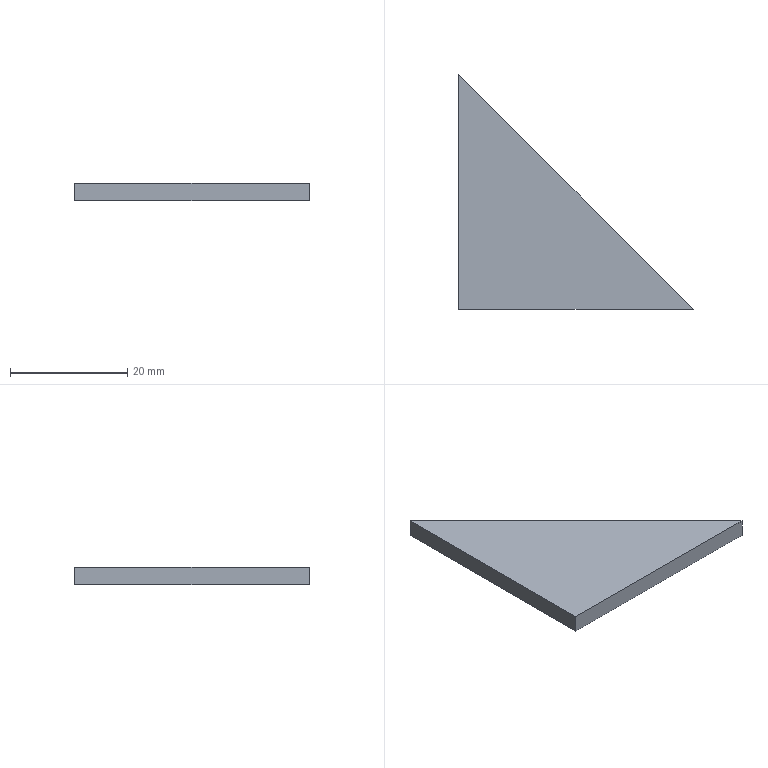Part | STEP file | 7100107 | 1 solid | 5 faces | box 40 x 40 x 3 mm | volume 2400 mm3 | plane 5
STEP:
#1=CARTESIAN_POINT('',(0.,0.,0.));
#2=DIRECTION('',(0.,0.,1.));
#3=DIRECTION('',(1.,0.,0.));
#4=AXIS2_PLACEMENT_3D('',#1,#2,#3);
#5=CARTESIAN_POINT('',(40.,-40.,0.));
#6=VERTEX_POINT('',#5);
#7=CARTESIAN_POINT('',(0.,0.,0.));
#8=VERTEX_POINT('',#7);
#9=CARTESIAN_POINT('',(40.,-40.,0.));
#10=DIRECTION('',(-0.7071,0.7071,0.));
#11=VECTOR('',#10,1.);
#12=LINE('',#9,#11);
#13=CARTESIAN_POINT('',(40.,-40.,3.));
#14=DIRECTION('',(-0.7071,-0.7071,0.));
#15=DIRECTION('',(0.7071,-0.7071,0.));
#16=AXIS2_PLACEMENT_3D('',#13,#14,#15);
#17=PLANE('',#16);
#18=CARTESIAN_POINT('',(0.,-3.));
#19=DIRECTION('',(-1.,0.));
#20=VECTOR('',#19,1.);
#21=LINE('',#18,#20);
#22=(GEOMETRIC_REPRESENTATION_CONTEXT(2)PARAMETRIC_REPRESENTATION_CONTEXT()REPRESENTATION_CONTEXT('',''));
#23=DEFINITIONAL_REPRESENTATION('',(#21),#22);
#24=PCURVE('',#17,#23);
#25=CARTESIAN_POINT('',(0.,0.,0.));
#26=DIRECTION('',(0.,0.,1.));
#27=DIRECTION('',(1.,0.,0.));
#28=AXIS2_PLACEMENT_3D('',#25,#26,#27);
#29=PLANE('',#28);
#30=CARTESIAN_POINT('',(40.,-40.));
#31=DIRECTION('',(-0.7071,0.7071));
#32=VECTOR('',#31,1.);
#33=LINE('',#30,#32);
#34=(GEOMETRIC_REPRESENTATION_CONTEXT(2)PARAMETRIC_REPRESENTATION_CONTEXT()REPRESENTATION_CONTEXT('',''));
#35=DEFINITIONAL_REPRESENTATION('',(#33),#34);
#36=PCURVE('',#29,#35);
#37=SURFACE_CURVE('',#12,(#24,#36),.PCURVE_S1.);
#38=EDGE_CURVE('',#6,#8,#37,.T.);
#39=ORIENTED_EDGE('',*,*,#38,.T.);
#40=CARTESIAN_POINT('',(0.,0.,3.));
#41=VERTEX_POINT('',#40);
#42=CARTESIAN_POINT('',(0.,0.,3.));
#43=DIRECTION('',(0.,0.,-1.));
#44=VECTOR('',#43,1.);
#45=LINE('',#42,#44);
#46=CARTESIAN_POINT('',(-56.569,0.));
#47=DIRECTION('',(0.,-1.));
#48=VECTOR('',#47,1.);
#49=LINE('',#46,#48);
#50=(GEOMETRIC_REPRESENTATION_CONTEXT(2)PARAMETRIC_REPRESENTATION_CONTEXT()REPRESENTATION_CONTEXT('',''));
#51=DEFINITIONAL_REPRESENTATION('',(#49),#50);
#52=PCURVE('',#17,#51);
#53=CARTESIAN_POINT('',(0.,0.,3.));
#54=DIRECTION('',(1.,0.,0.));
#55=DIRECTION('',(0.,1.,0.));
#56=AXIS2_PLACEMENT_3D('',#53,#54,#55);
#57=PLANE('',#56);
#58=CARTESIAN_POINT('',(0.,0.));
#59=DIRECTION('',(0.,-1.));
#60=VECTOR('',#59,1.);
#61=LINE('',#58,#60);
#62=(GEOMETRIC_REPRESENTATION_CONTEXT(2)PARAMETRIC_REPRESENTATION_CONTEXT()REPRESENTATION_CONTEXT('',''));
#63=DEFINITIONAL_REPRESENTATION('',(#61),#62);
#64=PCURVE('',#57,#63);
#65=SURFACE_CURVE('',#45,(#52,#64),.PCURVE_S1.);
#66=EDGE_CURVE('',#41,#8,#65,.T.);
#67=ORIENTED_EDGE('',*,*,#66,.F.);
#68=CARTESIAN_POINT('',(40.,-40.,3.));
#69=VERTEX_POINT('',#68);
#70=CARTESIAN_POINT('',(40.,-40.,3.));
#71=DIRECTION('',(-0.7071,0.7071,0.));
#72=VECTOR('',#71,1.);
#73=LINE('',#70,#72);
#74=CARTESIAN_POINT('',(0.,0.));
#75=DIRECTION('',(-1.,0.));
#76=VECTOR('',#75,1.);
#77=LINE('',#74,#76);
#78=(GEOMETRIC_REPRESENTATION_CONTEXT(2)PARAMETRIC_REPRESENTATION_CONTEXT()REPRESENTATION_CONTEXT('',''));
#79=DEFINITIONAL_REPRESENTATION('',(#77),#78);
#80=PCURVE('',#17,#79);
#81=CARTESIAN_POINT('',(0.,0.,3.));
#82=DIRECTION('',(0.,0.,1.));
#83=DIRECTION('',(1.,0.,0.));
#84=AXIS2_PLACEMENT_3D('',#81,#82,#83);
#85=PLANE('',#84);
#86=CARTESIAN_POINT('',(40.,-40.));
#87=DIRECTION('',(-0.7071,0.7071));
#88=VECTOR('',#87,1.);
#89=LINE('',#86,#88);
#90=(GEOMETRIC_REPRESENTATION_CONTEXT(2)PARAMETRIC_REPRESENTATION_CONTEXT()REPRESENTATION_CONTEXT('',''));
#91=DEFINITIONAL_REPRESENTATION('',(#89),#90);
#92=PCURVE('',#85,#91);
#93=SURFACE_CURVE('',#73,(#80,#92),.PCURVE_S1.);
#94=EDGE_CURVE('',#69,#41,#93,.T.);
#95=ORIENTED_EDGE('',*,*,#94,.F.);
#96=CARTESIAN_POINT('',(40.,-40.,3.));
#97=DIRECTION('',(0.,0.,-1.));
#98=VECTOR('',#97,1.);
#99=LINE('',#96,#98);
#100=CARTESIAN_POINT('',(0.,0.));
#101=DIRECTION('',(0.,-1.));
#102=VECTOR('',#101,1.);
#103=LINE('',#100,#102);
#104=(GEOMETRIC_REPRESENTATION_CONTEXT(2)PARAMETRIC_REPRESENTATION_CONTEXT()REPRESENTATION_CONTEXT('',''));
#105=DEFINITIONAL_REPRESENTATION('',(#103),#104);
#106=PCURVE('',#17,#105);
#107=CARTESIAN_POINT('',(0.,-40.,3.));
#108=DIRECTION('',(0.,1.,0.));
#109=DIRECTION('',(0.,0.,1.));
#110=AXIS2_PLACEMENT_3D('',#107,#108,#109);
#111=PLANE('',#110);
#112=CARTESIAN_POINT('',(0.,40.));
#113=DIRECTION('',(-1.,0.));
#114=VECTOR('',#113,1.);
#115=LINE('',#112,#114);
#116=(GEOMETRIC_REPRESENTATION_CONTEXT(2)PARAMETRIC_REPRESENTATION_CONTEXT()REPRESENTATION_CONTEXT('',''));
#117=DEFINITIONAL_REPRESENTATION('',(#115),#116);
#118=PCURVE('',#111,#117);
#119=SURFACE_CURVE('',#99,(#106,#118),.PCURVE_S1.);
#120=EDGE_CURVE('',#69,#6,#119,.T.);
#121=ORIENTED_EDGE('',*,*,#120,.T.);
#122=EDGE_LOOP('',(#39,#67,#95,#121));
#123=FACE_BOUND('',#122,.T.);
#124=ADVANCED_FACE('',(#123),#17,.F.);
#125=CARTESIAN_POINT('',(0.,-40.,0.));
#126=VERTEX_POINT('',#125);
#127=CARTESIAN_POINT('',(0.,0.,0.));
#128=DIRECTION('',(0.,-1.,0.));
#129=VECTOR('',#128,1.);
#130=LINE('',#127,#129);
#131=CARTESIAN_POINT('',(0.,-3.));
#132=DIRECTION('',(-1.,0.));
#133=VECTOR('',#132,1.);
#134=LINE('',#131,#133);
#135=(GEOMETRIC_REPRESENTATION_CONTEXT(2)PARAMETRIC_REPRESENTATION_CONTEXT()REPRESENTATION_CONTEXT('',''));
#136=DEFINITIONAL_REPRESENTATION('',(#134),#135);
#137=PCURVE('',#57,#136);
#138=CARTESIAN_POINT('',(0.,0.));
#139=DIRECTION('',(0.,-1.));
#140=VECTOR('',#139,1.);
#141=LINE('',#138,#140);
#142=(GEOMETRIC_REPRESENTATION_CONTEXT(2)PARAMETRIC_REPRESENTATION_CONTEXT()REPRESENTATION_CONTEXT('',''));
#143=DEFINITIONAL_REPRESENTATION('',(#141),#142);
#144=PCURVE('',#29,#143);
#145=SURFACE_CURVE('',#130,(#137,#144),.PCURVE_S1.);
#146=EDGE_CURVE('',#8,#126,#145,.T.);
#147=ORIENTED_EDGE('',*,*,#146,.T.);
#148=CARTESIAN_POINT('',(0.,-40.,3.));
#149=VERTEX_POINT('',#148);
#150=CARTESIAN_POINT('',(0.,-40.,3.));
#151=DIRECTION('',(0.,0.,-1.));
#152=VECTOR('',#151,1.);
#153=LINE('',#150,#152);
#154=CARTESIAN_POINT('',(-40.,0.));
#155=DIRECTION('',(0.,-1.));
#156=VECTOR('',#155,1.);
#157=LINE('',#154,#156);
#158=(GEOMETRIC_REPRESENTATION_CONTEXT(2)PARAMETRIC_REPRESENTATION_CONTEXT()REPRESENTATION_CONTEXT('',''));
#159=DEFINITIONAL_REPRESENTATION('',(#157),#158);
#160=PCURVE('',#57,#159);
#161=CARTESIAN_POINT('',(0.,0.));
#162=DIRECTION('',(-1.,0.));
#163=VECTOR('',#162,1.);
#164=LINE('',#161,#163);
#165=(GEOMETRIC_REPRESENTATION_CONTEXT(2)PARAMETRIC_REPRESENTATION_CONTEXT()REPRESENTATION_CONTEXT('',''));
#166=DEFINITIONAL_REPRESENTATION('',(#164),#165);
#167=PCURVE('',#111,#166);
#168=SURFACE_CURVE('',#153,(#160,#167),.PCURVE_S1.);
#169=EDGE_CURVE('',#149,#126,#168,.T.);
#170=ORIENTED_EDGE('',*,*,#169,.F.);
#171=CARTESIAN_POINT('',(0.,0.,3.));
#172=DIRECTION('',(0.,-1.,0.));
#173=VECTOR('',#172,1.);
#174=LINE('',#171,#173);
#175=CARTESIAN_POINT('',(0.,0.));
#176=DIRECTION('',(-1.,0.));
#177=VECTOR('',#176,1.);
#178=LINE('',#175,#177);
#179=(GEOMETRIC_REPRESENTATION_CONTEXT(2)PARAMETRIC_REPRESENTATION_CONTEXT()REPRESENTATION_CONTEXT('',''));
#180=DEFINITIONAL_REPRESENTATION('',(#178),#179);
#181=PCURVE('',#57,#180);
#182=CARTESIAN_POINT('',(0.,0.));
#183=DIRECTION('',(0.,-1.));
#184=VECTOR('',#183,1.);
#185=LINE('',#182,#184);
#186=(GEOMETRIC_REPRESENTATION_CONTEXT(2)PARAMETRIC_REPRESENTATION_CONTEXT()REPRESENTATION_CONTEXT('',''));
#187=DEFINITIONAL_REPRESENTATION('',(#185),#186);
#188=PCURVE('',#85,#187);
#189=SURFACE_CURVE('',#174,(#181,#188),.PCURVE_S1.);
#190=EDGE_CURVE('',#41,#149,#189,.T.);
#191=ORIENTED_EDGE('',*,*,#190,.F.);
#192=ORIENTED_EDGE('',*,*,#66,.T.);
#193=EDGE_LOOP('',(#147,#170,#191,#192));
#194=FACE_BOUND('',#193,.T.);
#195=ADVANCED_FACE('',(#194),#57,.F.);
#196=CARTESIAN_POINT('',(0.,-40.,0.));
#197=DIRECTION('',(1.,0.,0.));
#198=VECTOR('',#197,1.);
#199=LINE('',#196,#198);
#200=CARTESIAN_POINT('',(-3.,0.));
#201=DIRECTION('',(0.,1.));
#202=VECTOR('',#201,1.);
#203=LINE('',#200,#202);
#204=(GEOMETRIC_REPRESENTATION_CONTEXT(2)PARAMETRIC_REPRESENTATION_CONTEXT()REPRESENTATION_CONTEXT('',''));
#205=DEFINITIONAL_REPRESENTATION('',(#203),#204);
#206=PCURVE('',#111,#205);
#207=CARTESIAN_POINT('',(0.,-40.));
#208=DIRECTION('',(1.,0.));
#209=VECTOR('',#208,1.);
#210=LINE('',#207,#209);
#211=(GEOMETRIC_REPRESENTATION_CONTEXT(2)PARAMETRIC_REPRESENTATION_CONTEXT()REPRESENTATION_CONTEXT('',''));
#212=DEFINITIONAL_REPRESENTATION('',(#210),#211);
#213=PCURVE('',#29,#212);
#214=SURFACE_CURVE('',#199,(#206,#213),.PCURVE_S1.);
#215=EDGE_CURVE('',#126,#6,#214,.T.);
#216=ORIENTED_EDGE('',*,*,#215,.T.);
#217=ORIENTED_EDGE('',*,*,#120,.F.);
#218=CARTESIAN_POINT('',(0.,-40.,3.));
#219=DIRECTION('',(1.,0.,0.));
#220=VECTOR('',#219,1.);
#221=LINE('',#218,#220);
#222=CARTESIAN_POINT('',(0.,0.));
#223=DIRECTION('',(0.,1.));
#224=VECTOR('',#223,1.);
#225=LINE('',#222,#224);
#226=(GEOMETRIC_REPRESENTATION_CONTEXT(2)PARAMETRIC_REPRESENTATION_CONTEXT()REPRESENTATION_CONTEXT('',''));
#227=DEFINITIONAL_REPRESENTATION('',(#225),#226);
#228=PCURVE('',#111,#227);
#229=CARTESIAN_POINT('',(0.,-40.));
#230=DIRECTION('',(1.,0.));
#231=VECTOR('',#230,1.);
#232=LINE('',#229,#231);
#233=(GEOMETRIC_REPRESENTATION_CONTEXT(2)PARAMETRIC_REPRESENTATION_CONTEXT()REPRESENTATION_CONTEXT('',''));
#234=DEFINITIONAL_REPRESENTATION('',(#232),#233);
#235=PCURVE('',#85,#234);
#236=SURFACE_CURVE('',#221,(#228,#235),.PCURVE_S1.);
#237=EDGE_CURVE('',#149,#69,#236,.T.);
#238=ORIENTED_EDGE('',*,*,#237,.F.);
#239=ORIENTED_EDGE('',*,*,#169,.T.);
#240=EDGE_LOOP('',(#216,#217,#238,#239));
#241=FACE_BOUND('',#240,.T.);
#242=ADVANCED_FACE('',(#241),#111,.F.);
#243=ORIENTED_EDGE('',*,*,#94,.T.);
#244=ORIENTED_EDGE('',*,*,#190,.T.);
#245=ORIENTED_EDGE('',*,*,#237,.T.);
#246=EDGE_LOOP('',(#243,#244,#245));
#247=FACE_BOUND('',#246,.T.);
#248=ADVANCED_FACE('',(#247),#85,.T.);
#249=ORIENTED_EDGE('',*,*,#38,.F.);
#250=ORIENTED_EDGE('',*,*,#215,.F.);
#251=ORIENTED_EDGE('',*,*,#146,.F.);
#252=EDGE_LOOP('',(#249,#250,#251));
#253=FACE_BOUND('',#252,.T.);
#254=ADVANCED_FACE('',(#253),#29,.F.);
#255=CLOSED_SHELL('',(#124,#195,#242,#248,#254));
#256=MANIFOLD_SOLID_BREP('',#255);
#257=(LENGTH_UNIT()NAMED_UNIT(*)SI_UNIT(.MILLI.,.METRE.));
#258=UNCERTAINTY_MEASURE_WITH_UNIT(LENGTH_MEASURE(0.0000001),#257,'','');
#259=(NAMED_UNIT(*)PLANE_ANGLE_UNIT()SI_UNIT($,.RADIAN.));
#260=(NAMED_UNIT(*)SI_UNIT($,.STERADIAN.)SOLID_ANGLE_UNIT());
#261=(GEOMETRIC_REPRESENTATION_CONTEXT(3)GLOBAL_UNCERTAINTY_ASSIGNED_CONTEXT((#258))GLOBAL_UNIT_ASSIGNED_CONTEXT((#257,#259,#260))REPRESENTATION_CONTEXT('',''));
#262=ADVANCED_BREP_SHAPE_REPRESENTATION('',(#4,#256),#261);